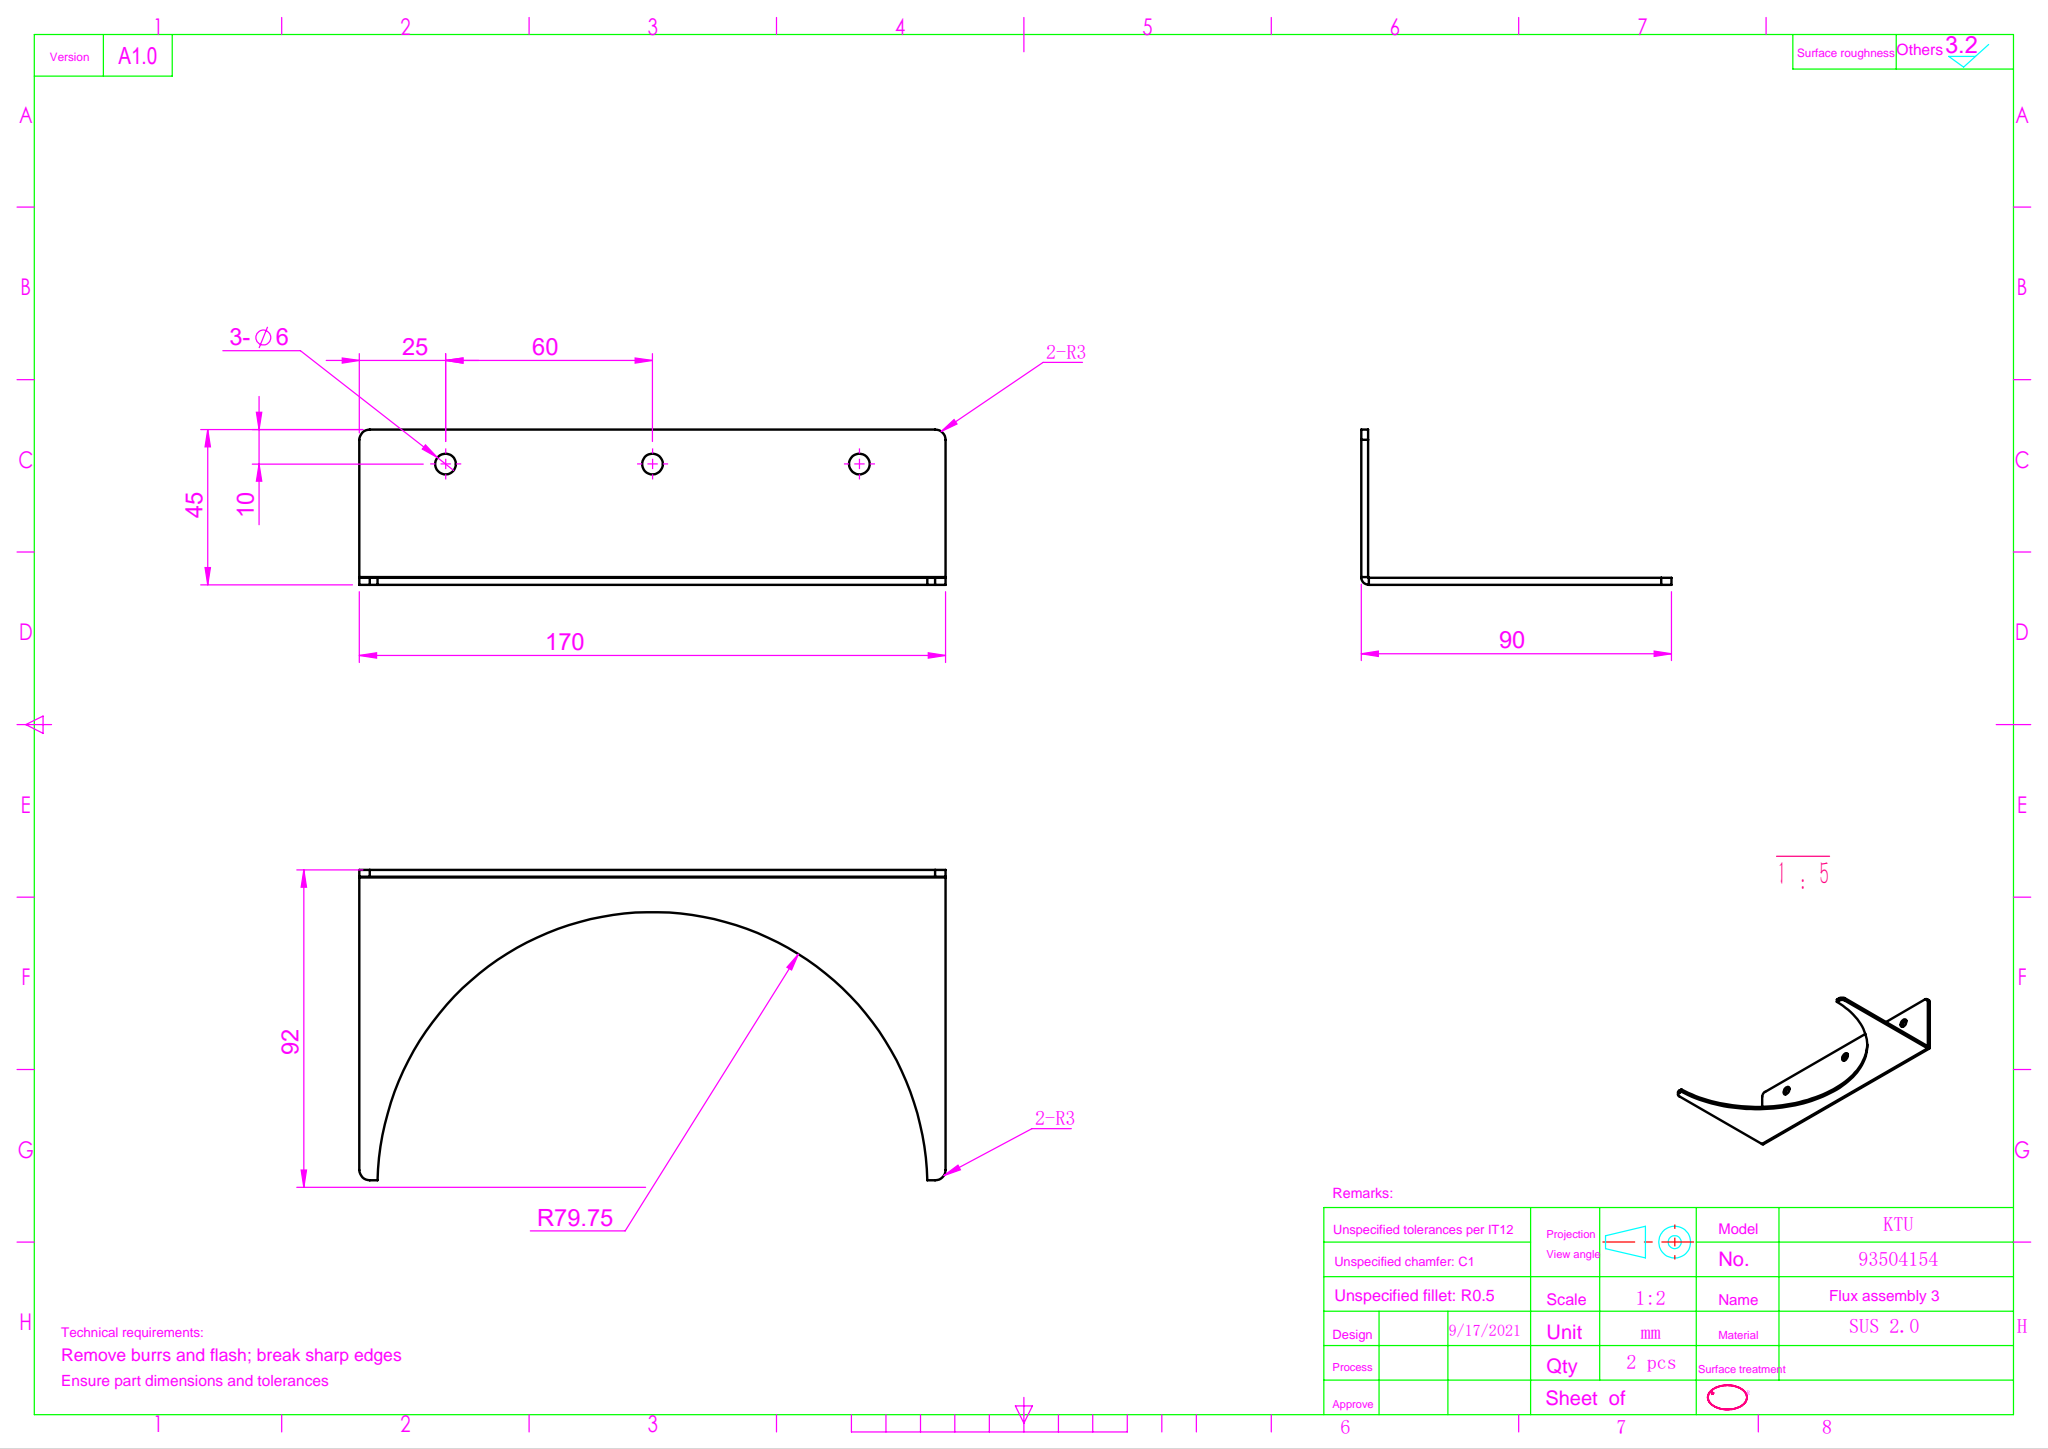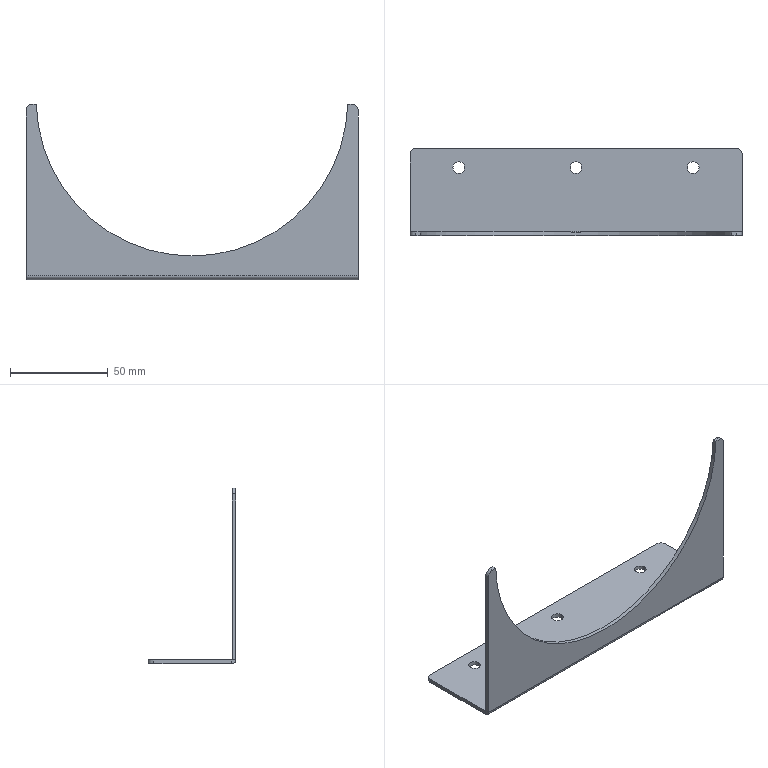Part | SolidWorks | features ICE 2, EdgeFlange 1, Fillet 1, FlatPattern 1, SMBaseFlange 1, SheetMetal 1 | 1 solid | 26 faces | box 170 x 45 x 90 mm | volume 25517 mm3 | cylinder 13 | plane 13 | commonest cylinder face diameters 6 x10 0.4 x1 4.4 x1 159.5 x1
STEP:
#1=CARTESIAN_POINT('',(-63.,33.,-92.));
#2=VERTEX_POINT('',#1);
#3=CARTESIAN_POINT('',(-57.,33.,-92.));
#4=VERTEX_POINT('',#3);
#5=CARTESIAN_POINT('',(-60.,33.,-92.));
#6=DIRECTION('',(0.,0.,1.));
#7=DIRECTION('',(1.,0.,0.));
#8=AXIS2_PLACEMENT_3D('',#5,#6,#7);
#9=CIRCLE('',#8,3.);
#10=EDGE_CURVE('',#2,#4,#9,.T.);
#11=ORIENTED_EDGE('',*,*,#10,.F.);
#12=CARTESIAN_POINT('',(-63.,33.,-90.));
#13=VERTEX_POINT('',#12);
#14=CARTESIAN_POINT('',(-63.,33.,-92.));
#15=DIRECTION('',(0.,0.,1.));
#16=VECTOR('',#15,1000.);
#17=LINE('',#14,#16);
#18=EDGE_CURVE('',#2,#13,#17,.T.);
#19=ORIENTED_EDGE('',*,*,#18,.T.);
#20=CARTESIAN_POINT('',(-57.,33.,-90.));
#21=VERTEX_POINT('',#20);
#22=CARTESIAN_POINT('',(-60.,33.,-90.));
#23=DIRECTION('',(0.,0.,1.));
#24=DIRECTION('',(1.,0.,0.));
#25=AXIS2_PLACEMENT_3D('',#22,#23,#24);
#26=CIRCLE('',#25,3.);
#27=EDGE_CURVE('',#13,#21,#26,.T.);
#28=ORIENTED_EDGE('',*,*,#27,.T.);
#29=CARTESIAN_POINT('',(-57.,33.,-92.));
#30=DIRECTION('',(0.,0.,1.));
#31=VECTOR('',#30,1000.);
#32=LINE('',#29,#31);
#33=EDGE_CURVE('',#4,#21,#32,.T.);
#34=ORIENTED_EDGE('',*,*,#33,.F.);
#35=EDGE_LOOP('',(#11,#19,#28,#34));
#36=FACE_OUTER_BOUND('',#35,.T.);
#37=CARTESIAN_POINT('',(-60.,33.,-92.));
#38=DIRECTION('',(0.,0.,1.));
#39=DIRECTION('',(1.,0.,0.));
#40=AXIS2_PLACEMENT_3D('',#37,#38,#39);
#41=CYLINDRICAL_SURFACE('',#40,3.);
#42=ADVANCED_FACE('',(#36),#41,.F.);
#43=CARTESIAN_POINT('',(57.,33.,-92.));
#44=VERTEX_POINT('',#43);
#45=CARTESIAN_POINT('',(63.,33.,-92.));
#46=VERTEX_POINT('',#45);
#47=CARTESIAN_POINT('',(60.,33.,-92.));
#48=DIRECTION('',(0.,0.,1.));
#49=DIRECTION('',(-1.,0.,0.));
#50=AXIS2_PLACEMENT_3D('',#47,#48,#49);
#51=CIRCLE('',#50,3.);
#52=EDGE_CURVE('',#44,#46,#51,.T.);
#53=ORIENTED_EDGE('',*,*,#52,.F.);
#54=CARTESIAN_POINT('',(57.,33.,-90.));
#55=VERTEX_POINT('',#54);
#56=CARTESIAN_POINT('',(57.,33.,-92.));
#57=DIRECTION('',(0.,0.,1.));
#58=VECTOR('',#57,1000.);
#59=LINE('',#56,#58);
#60=EDGE_CURVE('',#44,#55,#59,.T.);
#61=ORIENTED_EDGE('',*,*,#60,.T.);
#62=CARTESIAN_POINT('',(63.,33.,-90.));
#63=VERTEX_POINT('',#62);
#64=CARTESIAN_POINT('',(60.,33.,-90.));
#65=DIRECTION('',(0.,0.,1.));
#66=DIRECTION('',(-1.,0.,0.));
#67=AXIS2_PLACEMENT_3D('',#64,#65,#66);
#68=CIRCLE('',#67,3.);
#69=EDGE_CURVE('',#55,#63,#68,.T.);
#70=ORIENTED_EDGE('',*,*,#69,.T.);
#71=CARTESIAN_POINT('',(63.,33.,-92.));
#72=DIRECTION('',(0.,0.,1.));
#73=VECTOR('',#72,1000.);
#74=LINE('',#71,#73);
#75=EDGE_CURVE('',#46,#63,#74,.T.);
#76=ORIENTED_EDGE('',*,*,#75,.F.);
#77=EDGE_LOOP('',(#53,#61,#70,#76));
#78=FACE_OUTER_BOUND('',#77,.T.);
#79=CARTESIAN_POINT('',(60.,33.,-92.));
#80=DIRECTION('',(0.,0.,1.));
#81=DIRECTION('',(1.,0.,0.));
#82=AXIS2_PLACEMENT_3D('',#79,#80,#81);
#83=CYLINDRICAL_SURFACE('',#82,3.);
#84=ADVANCED_FACE('',(#78),#83,.F.);
#85=CARTESIAN_POINT('',(-3.,33.,-92.));
#86=VERTEX_POINT('',#85);
#87=CARTESIAN_POINT('',(3.,33.,-92.));
#88=VERTEX_POINT('',#87);
#89=CARTESIAN_POINT('',(0.,33.,-92.));
#90=DIRECTION('',(0.,0.,1.));
#91=DIRECTION('',(1.,0.,0.));
#92=AXIS2_PLACEMENT_3D('',#89,#90,#91);
#93=CIRCLE('',#92,3.);
#94=EDGE_CURVE('',#86,#88,#93,.T.);
#95=ORIENTED_EDGE('',*,*,#94,.F.);
#96=CARTESIAN_POINT('',(-3.,33.,-90.));
#97=VERTEX_POINT('',#96);
#98=CARTESIAN_POINT('',(-3.,33.,-92.));
#99=DIRECTION('',(0.,0.,1.));
#100=VECTOR('',#99,1000.);
#101=LINE('',#98,#100);
#102=EDGE_CURVE('',#86,#97,#101,.T.);
#103=ORIENTED_EDGE('',*,*,#102,.T.);
#104=CARTESIAN_POINT('',(3.,33.,-90.));
#105=VERTEX_POINT('',#104);
#106=CARTESIAN_POINT('',(0.,33.,-90.));
#107=DIRECTION('',(0.,0.,1.));
#108=DIRECTION('',(1.,0.,0.));
#109=AXIS2_PLACEMENT_3D('',#106,#107,#108);
#110=CIRCLE('',#109,3.);
#111=EDGE_CURVE('',#97,#105,#110,.T.);
#112=ORIENTED_EDGE('',*,*,#111,.T.);
#113=CARTESIAN_POINT('',(3.,33.,-92.));
#114=DIRECTION('',(0.,0.,1.));
#115=VECTOR('',#114,1000.);
#116=LINE('',#113,#115);
#117=EDGE_CURVE('',#88,#105,#116,.T.);
#118=ORIENTED_EDGE('',*,*,#117,.F.);
#119=EDGE_LOOP('',(#95,#103,#112,#118));
#120=FACE_OUTER_BOUND('',#119,.T.);
#121=CARTESIAN_POINT('',(0.,33.,-92.));
#122=DIRECTION('',(0.,0.,1.));
#123=DIRECTION('',(1.,0.,0.));
#124=AXIS2_PLACEMENT_3D('',#121,#122,#123);
#125=CYLINDRICAL_SURFACE('',#124,3.);
#126=ADVANCED_FACE('',(#120),#125,.F.);
#127=CARTESIAN_POINT('',(-85.,-2.,-89.8));
#128=VERTEX_POINT('',#127);
#129=CARTESIAN_POINT('',(-85.,-2.,-5.));
#130=VERTEX_POINT('',#129);
#131=CARTESIAN_POINT('',(-85.,-2.,0.));
#132=DIRECTION('',(0.,0.,1.));
#133=VECTOR('',#132,1000.);
#134=LINE('',#131,#133);
#135=EDGE_CURVE('',#128,#130,#134,.T.);
#136=ORIENTED_EDGE('',*,*,#135,.T.);
#137=CARTESIAN_POINT('',(-85.,0.,-5.));
#138=VERTEX_POINT('',#137);
#139=CARTESIAN_POINT('',(-85.,-2.,-5.));
#140=DIRECTION('',(0.,1.,0.));
#141=VECTOR('',#140,1000.);
#142=LINE('',#139,#141);
#143=EDGE_CURVE('',#130,#138,#142,.T.);
#144=ORIENTED_EDGE('',*,*,#143,.T.);
#145=CARTESIAN_POINT('',(-85.,0.,-89.8));
#146=VERTEX_POINT('',#145);
#147=CARTESIAN_POINT('',(-85.,0.,0.));
#148=DIRECTION('',(0.,0.,1.));
#149=VECTOR('',#148,1000.);
#150=LINE('',#147,#149);
#151=EDGE_CURVE('',#146,#138,#150,.T.);
#152=ORIENTED_EDGE('',*,*,#151,.F.);
#153=CARTESIAN_POINT('',(-85.,0.,-89.8));
#154=DIRECTION('',(0.,-1.,0.));
#155=VECTOR('',#154,1000.);
#156=LINE('',#153,#155);
#157=EDGE_CURVE('',#146,#128,#156,.T.);
#158=ORIENTED_EDGE('',*,*,#157,.T.);
#159=EDGE_LOOP('',(#136,#144,#152,#158));
#160=FACE_OUTER_BOUND('',#159,.T.);
#161=CARTESIAN_POINT('',(-85.,-2.,0.));
#162=DIRECTION('',(-1.,0.,0.));
#163=DIRECTION('',(0.,0.,1.));
#164=AXIS2_PLACEMENT_3D('',#161,#162,#163);
#165=PLANE('',#164);
#166=ADVANCED_FACE('',(#160),#165,.T.);
#167=CARTESIAN_POINT('',(-79.725,-2.,-2.));
#168=VERTEX_POINT('',#167);
#169=CARTESIAN_POINT('',(-82.,-2.,-2.));
#170=VERTEX_POINT('',#169);
#171=CARTESIAN_POINT('',(0.,-2.,-2.));
#172=DIRECTION('',(-1.,0.,0.));
#173=VECTOR('',#172,1000.);
#174=LINE('',#171,#173);
#175=EDGE_CURVE('',#168,#170,#174,.T.);
#176=ORIENTED_EDGE('',*,*,#175,.T.);
#177=CARTESIAN_POINT('',(-82.,-2.,-5.));
#178=DIRECTION('',(0.,-1.,0.));
#179=DIRECTION('',(0.,0.,1.));
#180=AXIS2_PLACEMENT_3D('',#177,#178,#179);
#181=CIRCLE('',#180,3.);
#182=EDGE_CURVE('',#170,#130,#181,.T.);
#183=ORIENTED_EDGE('',*,*,#182,.T.);
#184=ORIENTED_EDGE('',*,*,#135,.F.);
#185=CARTESIAN_POINT('',(85.,-2.,-89.8));
#186=VERTEX_POINT('',#185);
#187=CARTESIAN_POINT('',(-85.,-2.,-89.8));
#188=DIRECTION('',(1.,0.,0.));
#189=VECTOR('',#188,1000.);
#190=LINE('',#187,#189);
#191=EDGE_CURVE('',#128,#186,#190,.T.);
#192=ORIENTED_EDGE('',*,*,#191,.T.);
#193=CARTESIAN_POINT('',(85.,-2.,-5.));
#194=VERTEX_POINT('',#193);
#195=CARTESIAN_POINT('',(85.,-2.,-92.));
#196=DIRECTION('',(0.,0.,-1.));
#197=VECTOR('',#196,1000.);
#198=LINE('',#195,#197);
#199=EDGE_CURVE('',#194,#186,#198,.T.);
#200=ORIENTED_EDGE('',*,*,#199,.F.);
#201=CARTESIAN_POINT('',(82.,-2.,-2.));
#202=VERTEX_POINT('',#201);
#203=CARTESIAN_POINT('',(82.,-2.,-5.));
#204=DIRECTION('',(0.,-1.,0.));
#205=DIRECTION('',(0.,0.,1.));
#206=AXIS2_PLACEMENT_3D('',#203,#204,#205);
#207=CIRCLE('',#206,3.);
#208=EDGE_CURVE('',#194,#202,#207,.T.);
#209=ORIENTED_EDGE('',*,*,#208,.T.);
#210=CARTESIAN_POINT('',(79.725,-2.,-2.));
#211=VERTEX_POINT('',#210);
#212=CARTESIAN_POINT('',(0.,-2.,-2.));
#213=DIRECTION('',(-1.,0.,0.));
#214=VECTOR('',#213,1000.);
#215=LINE('',#212,#214);
#216=EDGE_CURVE('',#202,#211,#215,.T.);
#217=ORIENTED_EDGE('',*,*,#216,.T.);
#218=CARTESIAN_POINT('',(0.,-2.,0.));
#219=DIRECTION('',(0.,1.,0.));
#220=DIRECTION('',(0.,0.,1.));
#221=AXIS2_PLACEMENT_3D('',#218,#219,#220);
#222=CIRCLE('',#221,79.75);
#223=EDGE_CURVE('',#211,#168,#222,.T.);
#224=ORIENTED_EDGE('',*,*,#223,.T.);
#225=EDGE_LOOP('',(#176,#183,#184,#192,#200,#209,#217,#224));
#226=FACE_OUTER_BOUND('',#225,.T.);
#227=CARTESIAN_POINT('',(0.,-2.,0.));
#228=DIRECTION('',(0.,1.,0.));
#229=DIRECTION('',(0.,0.,1.));
#230=AXIS2_PLACEMENT_3D('',#227,#228,#229);
#231=PLANE('',#230);
#232=ADVANCED_FACE('',(#226),#231,.F.);
#233=ORIENTED_EDGE('',*,*,#151,.T.);
#234=CARTESIAN_POINT('',(-82.,0.,-2.));
#235=VERTEX_POINT('',#234);
#236=CARTESIAN_POINT('',(-82.,0.,-5.));
#237=DIRECTION('',(0.,1.,0.));
#238=DIRECTION('',(0.,0.,1.));
#239=AXIS2_PLACEMENT_3D('',#236,#237,#238);
#240=CIRCLE('',#239,3.);
#241=EDGE_CURVE('',#138,#235,#240,.T.);
#242=ORIENTED_EDGE('',*,*,#241,.T.);
#243=CARTESIAN_POINT('',(-79.725,0.,-2.));
#244=VERTEX_POINT('',#243);
#245=CARTESIAN_POINT('',(0.,0.,-2.));
#246=DIRECTION('',(-1.,0.,0.));
#247=VECTOR('',#246,1000.);
#248=LINE('',#245,#247);
#249=EDGE_CURVE('',#244,#235,#248,.T.);
#250=ORIENTED_EDGE('',*,*,#249,.F.);
#251=CARTESIAN_POINT('',(79.725,0.,-2.));
#252=VERTEX_POINT('',#251);
#253=CARTESIAN_POINT('',(0.,0.,0.));
#254=DIRECTION('',(0.,1.,0.));
#255=DIRECTION('',(0.,0.,1.));
#256=AXIS2_PLACEMENT_3D('',#253,#254,#255);
#257=CIRCLE('',#256,79.75);
#258=EDGE_CURVE('',#252,#244,#257,.T.);
#259=ORIENTED_EDGE('',*,*,#258,.F.);
#260=CARTESIAN_POINT('',(82.,0.,-2.));
#261=VERTEX_POINT('',#260);
#262=CARTESIAN_POINT('',(0.,0.,-2.));
#263=DIRECTION('',(-1.,0.,0.));
#264=VECTOR('',#263,1000.);
#265=LINE('',#262,#264);
#266=EDGE_CURVE('',#261,#252,#265,.T.);
#267=ORIENTED_EDGE('',*,*,#266,.F.);
#268=CARTESIAN_POINT('',(85.,0.,-5.));
#269=VERTEX_POINT('',#268);
#270=CARTESIAN_POINT('',(82.,0.,-5.));
#271=DIRECTION('',(0.,1.,0.));
#272=DIRECTION('',(0.,0.,1.));
#273=AXIS2_PLACEMENT_3D('',#270,#271,#272);
#274=CIRCLE('',#273,3.);
#275=EDGE_CURVE('',#261,#269,#274,.T.);
#276=ORIENTED_EDGE('',*,*,#275,.T.);
#277=CARTESIAN_POINT('',(85.,0.,-89.8));
#278=VERTEX_POINT('',#277);
#279=CARTESIAN_POINT('',(85.,0.,-92.));
#280=DIRECTION('',(0.,0.,-1.));
#281=VECTOR('',#280,1000.);
#282=LINE('',#279,#281);
#283=EDGE_CURVE('',#269,#278,#282,.T.);
#284=ORIENTED_EDGE('',*,*,#283,.T.);
#285=CARTESIAN_POINT('',(-85.,0.,-89.8));
#286=DIRECTION('',(1.,0.,0.));
#287=VECTOR('',#286,1000.);
#288=LINE('',#285,#287);
#289=EDGE_CURVE('',#146,#278,#288,.T.);
#290=ORIENTED_EDGE('',*,*,#289,.F.);
#291=EDGE_LOOP('',(#233,#242,#250,#259,#267,#276,#284,#290));
#292=FACE_OUTER_BOUND('',#291,.T.);
#293=CARTESIAN_POINT('',(0.,0.,0.));
#294=DIRECTION('',(0.,1.,0.));
#295=DIRECTION('',(0.,0.,1.));
#296=AXIS2_PLACEMENT_3D('',#293,#294,#295);
#297=PLANE('',#296);
#298=ADVANCED_FACE('',(#292),#297,.T.);
#299=ORIENTED_EDGE('',*,*,#283,.F.);
#300=CARTESIAN_POINT('',(85.,-2.,-5.));
#301=DIRECTION('',(0.,-1.,0.));
#302=VECTOR('',#301,1000.);
#303=LINE('',#300,#302);
#304=EDGE_CURVE('',#269,#194,#303,.T.);
#305=ORIENTED_EDGE('',*,*,#304,.T.);
#306=ORIENTED_EDGE('',*,*,#199,.T.);
#307=CARTESIAN_POINT('',(85.,0.,-89.8));
#308=DIRECTION('',(0.,-1.,0.));
#309=VECTOR('',#308,1000.);
#310=LINE('',#307,#309);
#311=EDGE_CURVE('',#278,#186,#310,.T.);
#312=ORIENTED_EDGE('',*,*,#311,.F.);
#313=EDGE_LOOP('',(#299,#305,#306,#312));
#314=FACE_OUTER_BOUND('',#313,.T.);
#315=CARTESIAN_POINT('',(85.,-2.,-92.));
#316=DIRECTION('',(1.,0.,0.));
#317=DIRECTION('',(0.,0.,-1.));
#318=AXIS2_PLACEMENT_3D('',#315,#316,#317);
#319=PLANE('',#318);
#320=ADVANCED_FACE('',(#314),#319,.T.);
#321=CARTESIAN_POINT('',(-79.725,0.,-2.));
#322=DIRECTION('',(0.,-1.,0.));
#323=VECTOR('',#322,1000.);
#324=LINE('',#321,#323);
#325=EDGE_CURVE('',#244,#168,#324,.T.);
#326=ORIENTED_EDGE('',*,*,#325,.T.);
#327=ORIENTED_EDGE('',*,*,#223,.F.);
#328=CARTESIAN_POINT('',(79.725,0.,-2.));
#329=DIRECTION('',(0.,-1.,0.));
#330=VECTOR('',#329,1000.);
#331=LINE('',#328,#330);
#332=EDGE_CURVE('',#252,#211,#331,.T.);
#333=ORIENTED_EDGE('',*,*,#332,.F.);
#334=ORIENTED_EDGE('',*,*,#258,.T.);
#335=EDGE_LOOP('',(#326,#327,#333,#334));
#336=FACE_OUTER_BOUND('',#335,.T.);
#337=CARTESIAN_POINT('',(0.,-2.,0.));
#338=DIRECTION('',(0.,1.,0.));
#339=DIRECTION('',(0.,0.,1.));
#340=AXIS2_PLACEMENT_3D('',#337,#338,#339);
#341=CYLINDRICAL_SURFACE('',#340,79.75);
#342=ADVANCED_FACE('',(#336),#341,.F.);
#343=CARTESIAN_POINT('',(85.,0.2,-90.));
#344=VERTEX_POINT('',#343);
#345=CARTESIAN_POINT('',(85.,0.2,-92.));
#346=VERTEX_POINT('',#345);
#347=CARTESIAN_POINT('',(85.,0.2,-92.));
#348=DIRECTION('',(0.,0.,-1.));
#349=VECTOR('',#348,1000.);
#350=LINE('',#347,#349);
#351=EDGE_CURVE('',#344,#346,#350,.T.);
#352=ORIENTED_EDGE('',*,*,#351,.F.);
#353=CARTESIAN_POINT('',(85.,0.2,-89.8));
#354=DIRECTION('',(1.,0.,0.));
#355=DIRECTION('',(0.,-1.,0.));
#356=AXIS2_PLACEMENT_3D('',#353,#354,#355);
#357=CIRCLE('',#356,0.2);
#358=EDGE_CURVE('',#278,#344,#357,.T.);
#359=ORIENTED_EDGE('',*,*,#358,.F.);
#360=ORIENTED_EDGE('',*,*,#311,.T.);
#361=CARTESIAN_POINT('',(85.,0.2,-89.8));
#362=DIRECTION('',(1.,0.,0.));
#363=DIRECTION('',(0.,-1.,0.));
#364=AXIS2_PLACEMENT_3D('',#361,#362,#363);
#365=CIRCLE('',#364,2.2);
#366=EDGE_CURVE('',#186,#346,#365,.T.);
#367=ORIENTED_EDGE('',*,*,#366,.T.);
#368=EDGE_LOOP('',(#352,#359,#360,#367));
#369=FACE_OUTER_BOUND('',#368,.T.);
#370=CARTESIAN_POINT('',(85.,0.2,-89.8));
#371=DIRECTION('',(1.,0.,0.));
#372=DIRECTION('',(0.,1.,0.));
#373=AXIS2_PLACEMENT_3D('',#370,#371,#372);
#374=PLANE('',#373);
#375=ADVANCED_FACE('',(#369),#374,.T.);
#376=CARTESIAN_POINT('',(-85.,0.2,-90.));
#377=VERTEX_POINT('',#376);
#378=CARTESIAN_POINT('',(-85.,0.2,-89.8));
#379=DIRECTION('',(-1.,0.,0.));
#380=DIRECTION('',(0.,-1.,0.));
#381=AXIS2_PLACEMENT_3D('',#378,#379,#380);
#382=CIRCLE('',#381,0.2);
#383=EDGE_CURVE('',#377,#146,#382,.T.);
#384=ORIENTED_EDGE('',*,*,#383,.F.);
#385=CARTESIAN_POINT('',(-85.,0.2,-92.));
#386=VERTEX_POINT('',#385);
#387=CARTESIAN_POINT('',(-85.,0.2,-90.));
#388=DIRECTION('',(0.,0.,-1.));
#389=VECTOR('',#388,1000.);
#390=LINE('',#387,#389);
#391=EDGE_CURVE('',#377,#386,#390,.T.);
#392=ORIENTED_EDGE('',*,*,#391,.T.);
#393=CARTESIAN_POINT('',(-85.,0.2,-89.8));
#394=DIRECTION('',(-1.,0.,0.));
#395=DIRECTION('',(0.,-1.,0.));
#396=AXIS2_PLACEMENT_3D('',#393,#394,#395);
#397=CIRCLE('',#396,2.2);
#398=EDGE_CURVE('',#386,#128,#397,.T.);
#399=ORIENTED_EDGE('',*,*,#398,.T.);
#400=ORIENTED_EDGE('',*,*,#157,.F.);
#401=EDGE_LOOP('',(#384,#392,#399,#400));
#402=FACE_OUTER_BOUND('',#401,.T.);
#403=CARTESIAN_POINT('',(-85.,0.2,-89.8));
#404=DIRECTION('',(1.,0.,0.));
#405=DIRECTION('',(0.,1.,0.));
#406=AXIS2_PLACEMENT_3D('',#403,#404,#405);
#407=PLANE('',#406);
#408=ADVANCED_FACE('',(#402),#407,.F.);
#409=ORIENTED_EDGE('',*,*,#191,.F.);
#410=ORIENTED_EDGE('',*,*,#398,.F.);
#411=CARTESIAN_POINT('',(85.,0.2,-92.));
#412=DIRECTION('',(1.,0.,0.));
#413=VECTOR('',#412,1000.);
#414=LINE('',#411,#413);
#415=EDGE_CURVE('',#386,#346,#414,.T.);
#416=ORIENTED_EDGE('',*,*,#415,.T.);
#417=ORIENTED_EDGE('',*,*,#366,.F.);
#418=EDGE_LOOP('',(#409,#410,#416,#417));
#419=FACE_OUTER_BOUND('',#418,.T.);
#420=CARTESIAN_POINT('',(-85.,0.2,-89.8));
#421=DIRECTION('',(-1.,0.,0.));
#422=DIRECTION('',(0.,0.,-1.));
#423=AXIS2_PLACEMENT_3D('',#420,#421,#422);
#424=CYLINDRICAL_SURFACE('',#423,2.2);
#425=ADVANCED_FACE('',(#419),#424,.T.);
#426=ORIENTED_EDGE('',*,*,#289,.T.);
#427=ORIENTED_EDGE('',*,*,#358,.T.);
#428=CARTESIAN_POINT('',(85.,0.2,-90.));
#429=DIRECTION('',(-1.,0.,0.));
#430=VECTOR('',#429,1000.);
#431=LINE('',#428,#430);
#432=EDGE_CURVE('',#344,#377,#431,.T.);
#433=ORIENTED_EDGE('',*,*,#432,.T.);
#434=ORIENTED_EDGE('',*,*,#383,.T.);
#435=EDGE_LOOP('',(#426,#427,#433,#434));
#436=FACE_OUTER_BOUND('',#435,.T.);
#437=CARTESIAN_POINT('',(-85.,0.2,-89.8));
#438=DIRECTION('',(-1.,0.,0.));
#439=DIRECTION('',(0.,0.,-1.));
#440=AXIS2_PLACEMENT_3D('',#437,#438,#439);
#441=CYLINDRICAL_SURFACE('',#440,0.2);
#442=ADVANCED_FACE('',(#436),#441,.F.);
#443=CARTESIAN_POINT('',(85.,40.,-92.));
#444=VERTEX_POINT('',#443);
#445=CARTESIAN_POINT('',(85.,0.,-92.));
#446=DIRECTION('',(0.,-1.,0.));
#447=VECTOR('',#446,1000.);
#448=LINE('',#445,#447);
#449=EDGE_CURVE('',#444,#346,#448,.T.);
#450=ORIENTED_EDGE('',*,*,#449,.F.);
#451=CARTESIAN_POINT('',(85.,40.,-90.));
#452=VERTEX_POINT('',#451);
#453=CARTESIAN_POINT('',(85.,40.,-92.));
#454=DIRECTION('',(0.,0.,1.));
#455=VECTOR('',#454,1000.);
#456=LINE('',#453,#455);
#457=EDGE_CURVE('',#444,#452,#456,.T.);
#458=ORIENTED_EDGE('',*,*,#457,.T.);
#459=CARTESIAN_POINT('',(85.,0.,-90.));
#460=DIRECTION('',(0.,-1.,0.));
#461=VECTOR('',#460,1000.);
#462=LINE('',#459,#461);
#463=EDGE_CURVE('',#452,#344,#462,.T.);
#464=ORIENTED_EDGE('',*,*,#463,.T.);
#465=ORIENTED_EDGE('',*,*,#351,.T.);
#466=EDGE_LOOP('',(#450,#458,#464,#465));
#467=FACE_OUTER_BOUND('',#466,.T.);
#468=CARTESIAN_POINT('',(85.,0.,-92.));
#469=DIRECTION('',(-1.,0.,0.));
#470=DIRECTION('',(0.,0.,1.));
#471=AXIS2_PLACEMENT_3D('',#468,#469,#470);
#472=PLANE('',#471);
#473=ADVANCED_FACE('',(#467),#472,.F.);
#474=CARTESIAN_POINT('',(-85.,40.,-90.));
#475=VERTEX_POINT('',#474);
#476=CARTESIAN_POINT('',(-85.,43.,-90.));
#477=DIRECTION('',(0.,1.,0.));
#478=VECTOR('',#477,1000.);
#479=LINE('',#476,#478);
#480=EDGE_CURVE('',#377,#475,#479,.T.);
#481=ORIENTED_EDGE('',*,*,#480,.T.);
#482=CARTESIAN_POINT('',(-85.,40.,-92.));
#483=VERTEX_POINT('',#482);
#484=CARTESIAN_POINT('',(-85.,40.,-92.));
#485=DIRECTION('',(0.,0.,-1.));
#486=VECTOR('',#485,1000.);
#487=LINE('',#484,#486);
#488=EDGE_CURVE('',#475,#483,#487,.T.);
#489=ORIENTED_EDGE('',*,*,#488,.T.);
#490=CARTESIAN_POINT('',(-85.,0.,-92.));
#491=DIRECTION('',(0.,1.,0.));
#492=VECTOR('',#491,1000.);
#493=LINE('',#490,#492);
#494=EDGE_CURVE('',#386,#483,#493,.T.);
#495=ORIENTED_EDGE('',*,*,#494,.F.);
#496=ORIENTED_EDGE('',*,*,#391,.F.);
#497=EDGE_LOOP('',(#481,#489,#495,#496));
#498=FACE_OUTER_BOUND('',#497,.T.);
#499=CARTESIAN_POINT('',(-85.,43.,-92.));
#500=DIRECTION('',(1.,0.,0.));
#501=DIRECTION('',(0.,0.,-1.));
#502=AXIS2_PLACEMENT_3D('',#499,#500,#501);
#503=PLANE('',#502);
#504=ADVANCED_FACE('',(#498),#503,.F.);
#505=CARTESIAN_POINT('',(-60.,33.,-92.));
#506=DIRECTION('',(0.,0.,1.));
#507=DIRECTION('',(1.,0.,0.));
#508=AXIS2_PLACEMENT_3D('',#505,#506,#507);
#509=CIRCLE('',#508,3.);
#510=EDGE_CURVE('',#4,#2,#509,.T.);
#511=ORIENTED_EDGE('',*,*,#510,.T.);
#512=ORIENTED_EDGE('',*,*,#10,.T.);
#513=EDGE_LOOP('',(#511,#512));
#514=FACE_BOUND('',#513,.T.);
#515=CARTESIAN_POINT('',(60.,33.,-92.));
#516=DIRECTION('',(0.,0.,1.));
#517=DIRECTION('',(-1.,0.,0.));
#518=AXIS2_PLACEMENT_3D('',#515,#516,#517);
#519=CIRCLE('',#518,3.);
#520=EDGE_CURVE('',#46,#44,#519,.T.);
#521=ORIENTED_EDGE('',*,*,#520,.T.);
#522=ORIENTED_EDGE('',*,*,#52,.T.);
#523=EDGE_LOOP('',(#521,#522));
#524=FACE_BOUND('',#523,.T.);
#525=CARTESIAN_POINT('',(0.,33.,-92.));
#526=DIRECTION('',(0.,0.,1.));
#527=DIRECTION('',(1.,0.,0.));
#528=AXIS2_PLACEMENT_3D('',#525,#526,#527);
#529=CIRCLE('',#528,3.);
#530=EDGE_CURVE('',#88,#86,#529,.T.);
#531=ORIENTED_EDGE('',*,*,#530,.T.);
#532=ORIENTED_EDGE('',*,*,#94,.T.);
#533=EDGE_LOOP('',(#531,#532));
#534=FACE_BOUND('',#533,.T.);
#535=ORIENTED_EDGE('',*,*,#494,.T.);
#536=CARTESIAN_POINT('',(-82.,43.,-92.));
#537=VERTEX_POINT('',#536);
#538=CARTESIAN_POINT('',(-82.,40.,-92.));
#539=DIRECTION('',(0.,0.,-1.));
#540=DIRECTION('',(0.,-1.,0.));
#541=AXIS2_PLACEMENT_3D('',#538,#539,#540);
#542=CIRCLE('',#541,3.);
#543=EDGE_CURVE('',#483,#537,#542,.T.);
#544=ORIENTED_EDGE('',*,*,#543,.T.);
#545=CARTESIAN_POINT('',(82.,43.,-92.));
#546=VERTEX_POINT('',#545);
#547=CARTESIAN_POINT('',(0.,43.,-92.));
#548=DIRECTION('',(1.,0.,0.));
#549=VECTOR('',#548,1000.);
#550=LINE('',#547,#549);
#551=EDGE_CURVE('',#537,#546,#550,.T.);
#552=ORIENTED_EDGE('',*,*,#551,.T.);
#553=CARTESIAN_POINT('',(82.,40.,-92.));
#554=DIRECTION('',(0.,0.,-1.));
#555=DIRECTION('',(0.,-1.,0.));
#556=AXIS2_PLACEMENT_3D('',#553,#554,#555);
#557=CIRCLE('',#556,3.);
#558=EDGE_CURVE('',#546,#444,#557,.T.);
#559=ORIENTED_EDGE('',*,*,#558,.T.);
#560=ORIENTED_EDGE('',*,*,#449,.T.);
#561=ORIENTED_EDGE('',*,*,#415,.F.);
#562=EDGE_LOOP('',(#535,#544,#552,#559,#560,#561));
#563=FACE_OUTER_BOUND('',#562,.T.);
#564=CARTESIAN_POINT('',(0.,0.,-92.));
#565=DIRECTION('',(0.,0.,1.));
#566=DIRECTION('',(0.,-1.,0.));
#567=AXIS2_PLACEMENT_3D('',#564,#565,#566);
#568=PLANE('',#567);
#569=ADVANCED_FACE('',(#514,#524,#534,#563),#568,.F.);
#570=CARTESIAN_POINT('',(-60.,33.,-90.));
#571=DIRECTION('',(0.,0.,1.));
#572=DIRECTION('',(1.,0.,0.));
#573=AXIS2_PLACEMENT_3D('',#570,#571,#572);
#574=CIRCLE('',#573,3.);
#575=EDGE_CURVE('',#21,#13,#574,.T.);
#576=ORIENTED_EDGE('',*,*,#575,.F.);
#577=ORIENTED_EDGE('',*,*,#27,.F.);
#578=EDGE_LOOP('',(#576,#577));
#579=FACE_BOUND('',#578,.T.);
#580=CARTESIAN_POINT('',(60.,33.,-90.));
#581=DIRECTION('',(0.,0.,1.));
#582=DIRECTION('',(-1.,0.,0.));
#583=AXIS2_PLACEMENT_3D('',#580,#581,#582);
#584=CIRCLE('',#583,3.);
#585=EDGE_CURVE('',#63,#55,#584,.T.);
#586=ORIENTED_EDGE('',*,*,#585,.F.);
#587=ORIENTED_EDGE('',*,*,#69,.F.);
#588=EDGE_LOOP('',(#586,#587));
#589=FACE_BOUND('',#588,.T.);
#590=CARTESIAN_POINT('',(0.,33.,-90.));
#591=DIRECTION('',(0.,0.,1.));
#592=DIRECTION('',(1.,0.,0.));
#593=AXIS2_PLACEMENT_3D('',#590,#591,#592);
#594=CIRCLE('',#593,3.);
#595=EDGE_CURVE('',#105,#97,#594,.T.);
#596=ORIENTED_EDGE('',*,*,#595,.F.);
#597=ORIENTED_EDGE('',*,*,#111,.F.);
#598=EDGE_LOOP('',(#596,#597));
#599=FACE_BOUND('',#598,.T.);
#600=CARTESIAN_POINT('',(-82.,43.,-90.));
#601=VERTEX_POINT('',#600);
#602=CARTESIAN_POINT('',(82.,43.,-90.));
#603=VERTEX_POINT('',#602);
#604=CARTESIAN_POINT('',(85.,43.,-90.));
#605=DIRECTION('',(1.,0.,0.));
#606=VECTOR('',#605,1000.);
#607=LINE('',#604,#606);
#608=EDGE_CURVE('',#601,#603,#607,.T.);
#609=ORIENTED_EDGE('',*,*,#608,.F.);
#610=CARTESIAN_POINT('',(-82.,40.,-90.));
#611=DIRECTION('',(0.,0.,1.));
#612=DIRECTION('',(0.,-1.,0.));
#613=AXIS2_PLACEMENT_3D('',#610,#611,#612);
#614=CIRCLE('',#613,3.);
#615=EDGE_CURVE('',#601,#475,#614,.T.);
#616=ORIENTED_EDGE('',*,*,#615,.T.);
#617=ORIENTED_EDGE('',*,*,#480,.F.);
#618=ORIENTED_EDGE('',*,*,#432,.F.);
#619=ORIENTED_EDGE('',*,*,#463,.F.);
#620=CARTESIAN_POINT('',(82.,40.,-90.));
#621=DIRECTION('',(0.,0.,1.));
#622=DIRECTION('',(0.,-1.,0.));
#623=AXIS2_PLACEMENT_3D('',#620,#621,#622);
#624=CIRCLE('',#623,3.);
#625=EDGE_CURVE('',#452,#603,#624,.T.);
#626=ORIENTED_EDGE('',*,*,#625,.T.);
#627=EDGE_LOOP('',(#609,#616,#617,#618,#619,#626));
#628=FACE_OUTER_BOUND('',#627,.T.);
#629=CARTESIAN_POINT('',(0.,0.,-90.));
#630=DIRECTION('',(0.,0.,1.));
#631=DIRECTION('',(0.,-1.,0.));
#632=AXIS2_PLACEMENT_3D('',#629,#630,#631);
#633=PLANE('',#632);
#634=ADVANCED_FACE('',(#579,#589,#599,#628),#633,.T.);
#635=ORIENTED_EDGE('',*,*,#551,.F.);
#636=CARTESIAN_POINT('',(-82.,43.,-92.));
#637=DIRECTION('',(0.,0.,1.));
#638=VECTOR('',#637,1000.);
#639=LINE('',#636,#638);
#640=EDGE_CURVE('',#537,#601,#639,.T.);
#641=ORIENTED_EDGE('',*,*,#640,.T.);
#642=ORIENTED_EDGE('',*,*,#608,.T.);
#643=CARTESIAN_POINT('',(82.,43.,-92.));
#644=DIRECTION('',(0.,0.,-1.));
#645=VECTOR('',#644,1000.);
#646=LINE('',#643,#645);
#647=EDGE_CURVE('',#603,#546,#646,.T.);
#648=ORIENTED_EDGE('',*,*,#647,.T.);
#649=EDGE_LOOP('',(#635,#641,#642,#648));
#650=FACE_OUTER_BOUND('',#649,.T.);
#651=CARTESIAN_POINT('',(85.,43.,-92.));
#652=DIRECTION('',(0.,-1.,0.));
#653=DIRECTION('',(0.,0.,-1.));
#654=AXIS2_PLACEMENT_3D('',#651,#652,#653);
#655=PLANE('',#654);
#656=ADVANCED_FACE('',(#650),#655,.F.);
#657=ORIENTED_EDGE('',*,*,#102,.F.);
#658=ORIENTED_EDGE('',*,*,#530,.F.);
#659=ORIENTED_EDGE('',*,*,#117,.T.);
#660=ORIENTED_EDGE('',*,*,#595,.T.);
#661=EDGE_LOOP('',(#657,#658,#659,#660));
#662=FACE_OUTER_BOUND('',#661,.T.);
#663=CARTESIAN_POINT('',(0.,33.,-92.));
#664=DIRECTION('',(0.,0.,1.));
#665=DIRECTION('',(1.,0.,0.));
#666=AXIS2_PLACEMENT_3D('',#663,#664,#665);
#667=CYLINDRICAL_SURFACE('',#666,3.);
#668=ADVANCED_FACE('',(#662),#667,.F.);
#669=ORIENTED_EDGE('',*,*,#60,.F.);
#670=ORIENTED_EDGE('',*,*,#520,.F.);
#671=ORIENTED_EDGE('',*,*,#75,.T.);
#672=ORIENTED_EDGE('',*,*,#585,.T.);
#673=EDGE_LOOP('',(#669,#670,#671,#672));
#674=FACE_OUTER_BOUND('',#673,.T.);
#675=CARTESIAN_POINT('',(60.,33.,-92.));
#676=DIRECTION('',(0.,0.,1.));
#677=DIRECTION('',(1.,0.,0.));
#678=AXIS2_PLACEMENT_3D('',#675,#676,#677);
#679=CYLINDRICAL_SURFACE('',#678,3.);
#680=ADVANCED_FACE('',(#674),#679,.F.);
#681=ORIENTED_EDGE('',*,*,#18,.F.);
#682=ORIENTED_EDGE('',*,*,#510,.F.);
#683=ORIENTED_EDGE('',*,*,#33,.T.);
#684=ORIENTED_EDGE('',*,*,#575,.T.);
#685=EDGE_LOOP('',(#681,#682,#683,#684));
#686=FACE_OUTER_BOUND('',#685,.T.);
#687=CARTESIAN_POINT('',(-60.,33.,-92.));
#688=DIRECTION('',(0.,0.,1.));
#689=DIRECTION('',(1.,0.,0.));
#690=AXIS2_PLACEMENT_3D('',#687,#688,#689);
#691=CYLINDRICAL_SURFACE('',#690,3.);
#692=ADVANCED_FACE('',(#686),#691,.F.);
#693=ORIENTED_EDGE('',*,*,#216,.F.);
#694=CARTESIAN_POINT('',(82.,0.,-2.));
#695=DIRECTION('',(0.,1.,0.));
#696=VECTOR('',#695,1000.);
#697=LINE('',#694,#696);
#698=EDGE_CURVE('',#202,#261,#697,.T.);
#699=ORIENTED_EDGE('',*,*,#698,.T.);
#700=ORIENTED_EDGE('',*,*,#266,.T.);
#701=ORIENTED_EDGE('',*,*,#332,.T.);
#702=EDGE_LOOP('',(#693,#699,#700,#701));
#703=FACE_OUTER_BOUND('',#702,.T.);
#704=CARTESIAN_POINT('',(0.,0.,-2.));
#705=DIRECTION('',(0.,0.,-1.));
#706=DIRECTION('',(-1.,0.,0.));
#707=AXIS2_PLACEMENT_3D('',#704,#705,#706);
#708=PLANE('',#707);
#709=ADVANCED_FACE('',(#703),#708,.F.);
#710=ORIENTED_EDGE('',*,*,#249,.T.);
#711=CARTESIAN_POINT('',(-82.,0.,-2.));
#712=DIRECTION('',(0.,-1.,0.));
#713=VECTOR('',#712,1000.);
#714=LINE('',#711,#713);
#715=EDGE_CURVE('',#235,#170,#714,.T.);
#716=ORIENTED_EDGE('',*,*,#715,.T.);
#717=ORIENTED_EDGE('',*,*,#175,.F.);
#718=ORIENTED_EDGE('',*,*,#325,.F.);
#719=EDGE_LOOP('',(#710,#716,#717,#718));
#720=FACE_OUTER_BOUND('',#719,.T.);
#721=CARTESIAN_POINT('',(0.,0.,-2.));
#722=DIRECTION('',(0.,0.,-1.));
#723=DIRECTION('',(-1.,0.,0.));
#724=AXIS2_PLACEMENT_3D('',#721,#722,#723);
#725=PLANE('',#724);
#726=ADVANCED_FACE('',(#720),#725,.F.);
#727=ORIENTED_EDGE('',*,*,#241,.F.);
#728=ORIENTED_EDGE('',*,*,#143,.F.);
#729=ORIENTED_EDGE('',*,*,#182,.F.);
#730=ORIENTED_EDGE('',*,*,#715,.F.);
#731=EDGE_LOOP('',(#727,#728,#729,#730));
#732=FACE_OUTER_BOUND('',#731,.T.);
#733=CARTESIAN_POINT('',(-82.,0.,-5.));
#734=DIRECTION('',(0.,1.,0.));
#735=DIRECTION('',(0.,0.,1.));
#736=AXIS2_PLACEMENT_3D('',#733,#734,#735);
#737=CYLINDRICAL_SURFACE('',#736,3.);
#738=ADVANCED_FACE('',(#732),#737,.T.);
#739=ORIENTED_EDGE('',*,*,#275,.F.);
#740=ORIENTED_EDGE('',*,*,#698,.F.);
#741=ORIENTED_EDGE('',*,*,#208,.F.);
#742=ORIENTED_EDGE('',*,*,#304,.F.);
#743=EDGE_LOOP('',(#739,#740,#741,#742));
#744=FACE_OUTER_BOUND('',#743,.T.);
#745=CARTESIAN_POINT('',(82.,-2.,-5.));
#746=DIRECTION('',(0.,1.,0.));
#747=DIRECTION('',(0.,0.,1.));
#748=AXIS2_PLACEMENT_3D('',#745,#746,#747);
#749=CYLINDRICAL_SURFACE('',#748,3.);
#750=ADVANCED_FACE('',(#744),#749,.T.);
#751=ORIENTED_EDGE('',*,*,#543,.F.);
#752=ORIENTED_EDGE('',*,*,#488,.F.);
#753=ORIENTED_EDGE('',*,*,#615,.F.);
#754=ORIENTED_EDGE('',*,*,#640,.F.);
#755=EDGE_LOOP('',(#751,#752,#753,#754));
#756=FACE_OUTER_BOUND('',#755,.T.);
#757=CARTESIAN_POINT('',(-82.,40.,-92.));
#758=DIRECTION('',(0.,0.,1.));
#759=DIRECTION('',(0.,-1.,0.));
#760=AXIS2_PLACEMENT_3D('',#757,#758,#759);
#761=CYLINDRICAL_SURFACE('',#760,3.);
#762=ADVANCED_FACE('',(#756),#761,.T.);
#763=ORIENTED_EDGE('',*,*,#558,.F.);
#764=ORIENTED_EDGE('',*,*,#647,.F.);
#765=ORIENTED_EDGE('',*,*,#625,.F.);
#766=ORIENTED_EDGE('',*,*,#457,.F.);
#767=EDGE_LOOP('',(#763,#764,#765,#766));
#768=FACE_OUTER_BOUND('',#767,.T.);
#769=CARTESIAN_POINT('',(82.,40.,-92.));
#770=DIRECTION('',(0.,0.,1.));
#771=DIRECTION('',(0.,-1.,0.));
#772=AXIS2_PLACEMENT_3D('',#769,#770,#771);
#773=CYLINDRICAL_SURFACE('',#772,3.);
#774=ADVANCED_FACE('',(#768),#773,.T.);
#775=CLOSED_SHELL('',(#42,#84,#126,#166,#232,#298,#320,#342,#375,#408,#425,#442,#473,#504,#569,#634,#656,#668,#680,#692,#709,#726,#738,#750,#762,#774));
#776=MANIFOLD_SOLID_BREP('',#775);
#777=CARTESIAN_POINT('',(0.,0.,0.));
#778=DIRECTION('',(0.,0.,1.));
#779=DIRECTION('',(1.,0.,0.));
#780=AXIS2_PLACEMENT_3D('',#777,#778,#779);
#781=(LENGTH_UNIT()NAMED_UNIT(*)SI_UNIT(.MILLI.,.METRE.));
#782=UNCERTAINTY_MEASURE_WITH_UNIT(LENGTH_MEASURE(0.00001),#781,'','');
#783=(NAMED_UNIT(*)PLANE_ANGLE_UNIT()SI_UNIT($,.RADIAN.));
#784=(NAMED_UNIT(*)SI_UNIT($,.STERADIAN.)SOLID_ANGLE_UNIT());
#785=(GEOMETRIC_REPRESENTATION_CONTEXT(3)GLOBAL_UNCERTAINTY_ASSIGNED_CONTEXT((#782))GLOBAL_UNIT_ASSIGNED_CONTEXT((#781,#783,#784))REPRESENTATION_CONTEXT('',''));
#786=ADVANCED_BREP_SHAPE_REPRESENTATION('',(#776,#780),#785);